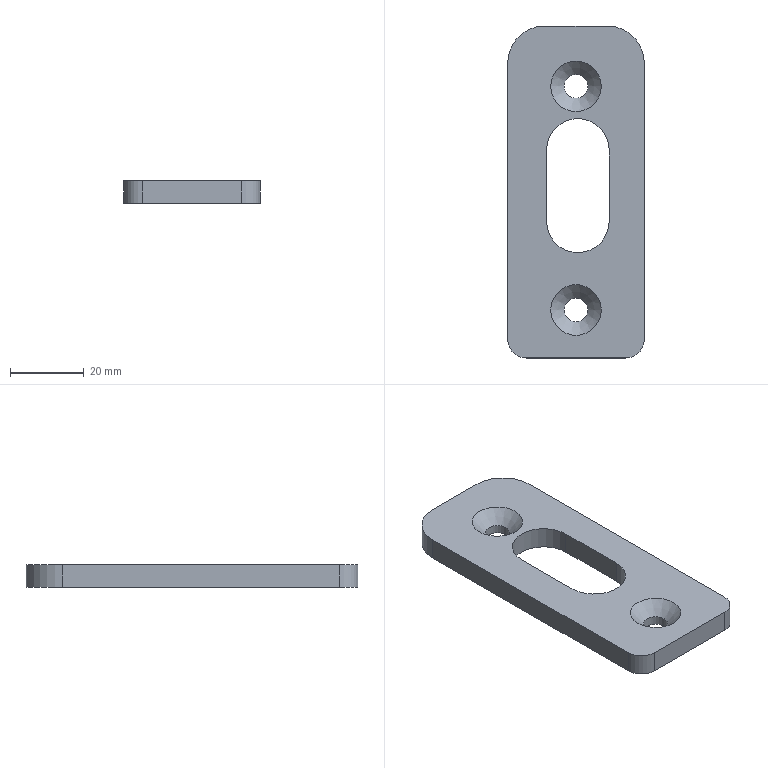Part | STEP file | solid 59 | 1 solid | 18 faces | box 37 x 90.006 x 6 mm | volume 15565 mm3 | plane 8 | cylinder 8 | cone 2 | commonest cylinder face diameters 6.5 x2 10 x2 17 x2 20 x2